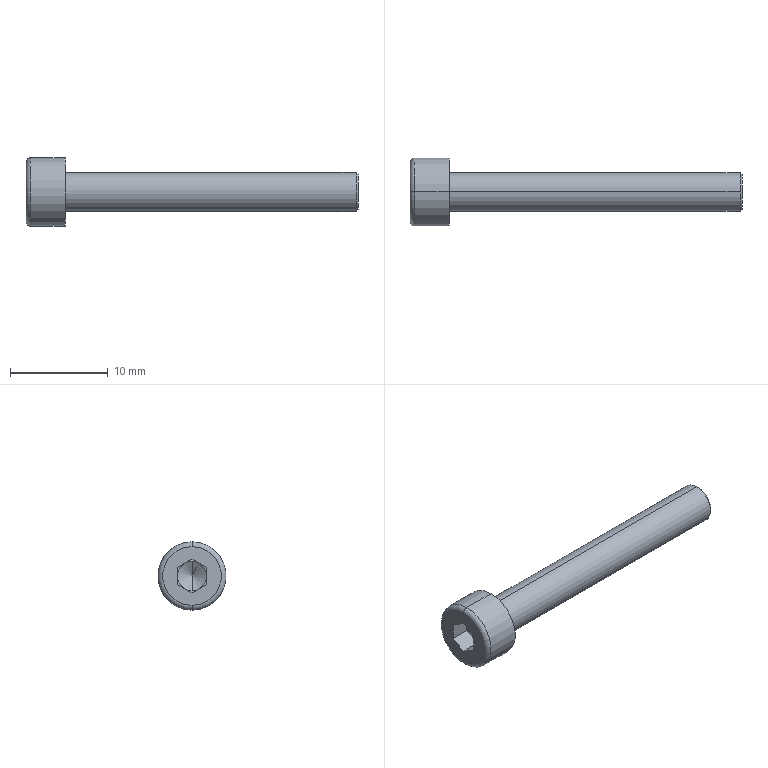Part | SolidWorks | features Fillet 2, RevCut 2, Boss 1, Chamfer 1, Cut 1, Extrusion 1, LPattern 1 | 1 solid | 25 faces | box 34 x 7 x 7 mm | volume 511.915 mm3 | plane 15 | cone 4 | cylinder 4 | torus 2 | commonest cylinder face diameters 4 x2 7 x2
STEP:
#1=CARTESIAN_POINT('',(34.,0.,-1.8));
#2=VERTEX_POINT('',#1);
#3=CARTESIAN_POINT('',(34.,0.,1.8));
#4=VERTEX_POINT('',#3);
#5=CARTESIAN_POINT('',(34.,0.,0.));
#6=DIRECTION('',(1.,0.,0.));
#7=DIRECTION('',(0.,0.,-1.));
#8=AXIS2_PLACEMENT_3D('',#5,#6,#7);
#9=CIRCLE('',#8,1.8);
#10=EDGE_CURVE('',#2,#4,#9,.T.);
#11=ORIENTED_EDGE('',*,*,#10,.F.);
#12=CARTESIAN_POINT('',(33.8,0.,-2.));
#13=VERTEX_POINT('',#12);
#14=CARTESIAN_POINT('',(34.,0.,-1.8));
#15=DIRECTION('',(-0.7071,0.,-0.7071));
#16=VECTOR('',#15,1000.);
#17=LINE('',#14,#16);
#18=EDGE_CURVE('',#2,#13,#17,.T.);
#19=ORIENTED_EDGE('',*,*,#18,.T.);
#20=CARTESIAN_POINT('',(33.8,0.,2.));
#21=VERTEX_POINT('',#20);
#22=CARTESIAN_POINT('',(33.8,0.,0.));
#23=DIRECTION('',(-1.,0.,0.));
#24=DIRECTION('',(0.,0.,-1.));
#25=AXIS2_PLACEMENT_3D('',#22,#23,#24);
#26=CIRCLE('',#25,2.);
#27=EDGE_CURVE('',#21,#13,#26,.T.);
#28=ORIENTED_EDGE('',*,*,#27,.F.);
#29=CARTESIAN_POINT('',(34.,0.,1.8));
#30=DIRECTION('',(-0.7071,0.,0.7071));
#31=VECTOR('',#30,1000.);
#32=LINE('',#29,#31);
#33=EDGE_CURVE('',#4,#21,#32,.T.);
#34=ORIENTED_EDGE('',*,*,#33,.F.);
#35=EDGE_LOOP('',(#11,#19,#28,#34));
#36=FACE_OUTER_BOUND('',#35,.T.);
#37=CARTESIAN_POINT('',(34.,0.,0.));
#38=DIRECTION('',(-1.,0.,0.));
#39=DIRECTION('',(0.,0.,1.));
#40=AXIS2_PLACEMENT_3D('',#37,#38,#39);
#41=CONICAL_SURFACE('',#40,1.8,0.7854);
#42=ADVANCED_FACE('',(#36),#41,.T.);
#43=CARTESIAN_POINT('',(0.,0.,3.));
#44=VERTEX_POINT('',#43);
#45=CARTESIAN_POINT('',(0.,0.,-3.));
#46=VERTEX_POINT('',#45);
#47=CARTESIAN_POINT('',(0.,0.,0.));
#48=DIRECTION('',(-1.,0.,0.));
#49=DIRECTION('',(0.,0.,-1.));
#50=AXIS2_PLACEMENT_3D('',#47,#48,#49);
#51=CIRCLE('',#50,3.);
#52=EDGE_CURVE('',#44,#46,#51,.T.);
#53=ORIENTED_EDGE('',*,*,#52,.F.);
#54=CARTESIAN_POINT('',(0.5,0.,3.5));
#55=VERTEX_POINT('',#54);
#56=CARTESIAN_POINT('',(0.5,0.,3.));
#57=DIRECTION('',(0.,1.,0.));
#58=DIRECTION('',(0.,0.,1.));
#59=AXIS2_PLACEMENT_3D('',#56,#57,#58);
#60=CIRCLE('',#59,0.5);
#61=EDGE_CURVE('',#44,#55,#60,.T.);
#62=ORIENTED_EDGE('',*,*,#61,.T.);
#63=CARTESIAN_POINT('',(0.5,0.,-3.5));
#64=VERTEX_POINT('',#63);
#65=CARTESIAN_POINT('',(0.5,0.,0.));
#66=DIRECTION('',(1.,0.,0.));
#67=DIRECTION('',(0.,0.,-1.));
#68=AXIS2_PLACEMENT_3D('',#65,#66,#67);
#69=CIRCLE('',#68,3.5);
#70=EDGE_CURVE('',#64,#55,#69,.T.);
#71=ORIENTED_EDGE('',*,*,#70,.F.);
#72=CARTESIAN_POINT('',(0.5,0.,-3.));
#73=DIRECTION('',(0.,-1.,0.));
#74=DIRECTION('',(0.,0.,-1.));
#75=AXIS2_PLACEMENT_3D('',#72,#73,#74);
#76=CIRCLE('',#75,0.5);
#77=EDGE_CURVE('',#46,#64,#76,.T.);
#78=ORIENTED_EDGE('',*,*,#77,.F.);
#79=EDGE_LOOP('',(#53,#62,#71,#78));
#80=FACE_OUTER_BOUND('',#79,.T.);
#81=CARTESIAN_POINT('',(0.5,0.,0.));
#82=DIRECTION('',(1.,0.,0.));
#83=DIRECTION('',(0.,0.,-1.));
#84=AXIS2_PLACEMENT_3D('',#81,#82,#83);
#85=TOROIDAL_SURFACE('',#84,3.,0.5);
#86=ADVANCED_FACE('',(#80),#85,.T.);
#87=CARTESIAN_POINT('',(2.866,0.,0.));
#88=VERTEX_POINT('',#87);
#89=CARTESIAN_POINT('',(2.,0.,1.5));
#90=VERTEX_POINT('',#89);
#91=CARTESIAN_POINT('',(2.,0.,1.5));
#92=DIRECTION('',(-0.5,0.,0.866));
#93=VECTOR('',#92,1000.);
#94=LINE('',#91,#93);
#95=EDGE_CURVE('',#88,#90,#94,.T.);
#96=ORIENTED_EDGE('',*,*,#95,.F.);
#97=CARTESIAN_POINT('',(2.,0.,-1.5));
#98=VERTEX_POINT('',#97);
#99=CARTESIAN_POINT('',(2.,0.,-1.5));
#100=DIRECTION('',(-0.5,0.,-0.866));
#101=VECTOR('',#100,1000.);
#102=LINE('',#99,#101);
#103=EDGE_CURVE('',#88,#98,#102,.T.);
#104=ORIENTED_EDGE('',*,*,#103,.T.);
#105=CARTESIAN_POINT('',(2.,-0.75,-1.299));
#106=VERTEX_POINT('',#105);
#107=CARTESIAN_POINT('',(2.,0.,0.));
#108=DIRECTION('',(-1.,0.,0.));
#109=DIRECTION('',(0.,0.,-1.));
#110=AXIS2_PLACEMENT_3D('',#107,#108,#109);
#111=CIRCLE('',#110,1.5);
#112=EDGE_CURVE('',#98,#106,#111,.T.);
#113=ORIENTED_EDGE('',*,*,#112,.T.);
#114=CARTESIAN_POINT('',(2.,-1.5,0.));
#115=VERTEX_POINT('',#114);
#116=CARTESIAN_POINT('',(2.,0.,0.));
#117=DIRECTION('',(-1.,0.,0.));
#118=DIRECTION('',(0.,0.,-1.));
#119=AXIS2_PLACEMENT_3D('',#116,#117,#118);
#120=CIRCLE('',#119,1.5);
#121=EDGE_CURVE('',#106,#115,#120,.T.);
#122=ORIENTED_EDGE('',*,*,#121,.T.);
#123=CARTESIAN_POINT('',(2.,-0.75,1.299));
#124=VERTEX_POINT('',#123);
#125=CARTESIAN_POINT('',(2.,0.,0.));
#126=DIRECTION('',(-1.,0.,0.));
#127=DIRECTION('',(0.,0.,-1.));
#128=AXIS2_PLACEMENT_3D('',#125,#126,#127);
#129=CIRCLE('',#128,1.5);
#130=EDGE_CURVE('',#115,#124,#129,.T.);
#131=ORIENTED_EDGE('',*,*,#130,.T.);
#132=CARTESIAN_POINT('',(2.,0.,0.));
#133=DIRECTION('',(-1.,0.,0.));
#134=DIRECTION('',(0.,0.,-1.));
#135=AXIS2_PLACEMENT_3D('',#132,#133,#134);
#136=CIRCLE('',#135,1.5);
#137=EDGE_CURVE('',#124,#90,#136,.T.);
#138=ORIENTED_EDGE('',*,*,#137,.T.);
#139=EDGE_LOOP('',(#96,#104,#113,#122,#131,#138));
#140=FACE_OUTER_BOUND('',#139,.T.);
#141=CARTESIAN_POINT('',(2.,0.,0.));
#142=DIRECTION('',(-1.,0.,0.));
#143=DIRECTION('',(0.,0.,1.));
#144=AXIS2_PLACEMENT_3D('',#141,#142,#143);
#145=CONICAL_SURFACE('',#144,1.5,1.047);
#146=ADVANCED_FACE('',(#140),#145,.F.);
#147=ORIENTED_EDGE('',*,*,#27,.T.);
#148=CARTESIAN_POINT('',(4.,0.,-2.));
#149=VERTEX_POINT('',#148);
#150=CARTESIAN_POINT('',(34.,0.,-2.));
#151=DIRECTION('',(-1.,0.,0.));
#152=VECTOR('',#151,1000.);
#153=LINE('',#150,#152);
#154=EDGE_CURVE('',#13,#149,#153,.T.);
#155=ORIENTED_EDGE('',*,*,#154,.T.);
#156=CARTESIAN_POINT('',(4.,0.,2.));
#157=VERTEX_POINT('',#156);
#158=CARTESIAN_POINT('',(4.,0.,0.));
#159=DIRECTION('',(1.,0.,0.));
#160=DIRECTION('',(0.,0.,-1.));
#161=AXIS2_PLACEMENT_3D('',#158,#159,#160);
#162=CIRCLE('',#161,2.);
#163=EDGE_CURVE('',#149,#157,#162,.T.);
#164=ORIENTED_EDGE('',*,*,#163,.T.);
#165=CARTESIAN_POINT('',(34.,0.,2.));
#166=DIRECTION('',(-1.,0.,0.));
#167=VECTOR('',#166,1000.);
#168=LINE('',#165,#167);
#169=EDGE_CURVE('',#21,#157,#168,.T.);
#170=ORIENTED_EDGE('',*,*,#169,.F.);
#171=EDGE_LOOP('',(#147,#155,#164,#170));
#172=FACE_OUTER_BOUND('',#171,.T.);
#173=CARTESIAN_POINT('',(34.,0.,0.));
#174=DIRECTION('',(-1.,0.,0.));
#175=DIRECTION('',(0.,0.,1.));
#176=AXIS2_PLACEMENT_3D('',#173,#174,#175);
#177=CYLINDRICAL_SURFACE('',#176,2.);
#178=ADVANCED_FACE('',(#172),#177,.T.);
#179=CARTESIAN_POINT('',(4.,0.,-3.5));
#180=VERTEX_POINT('',#179);
#181=CARTESIAN_POINT('',(4.,0.,3.5));
#182=VERTEX_POINT('',#181);
#183=CARTESIAN_POINT('',(4.,0.,0.));
#184=DIRECTION('',(1.,0.,0.));
#185=DIRECTION('',(0.,0.,-1.));
#186=AXIS2_PLACEMENT_3D('',#183,#184,#185);
#187=CIRCLE('',#186,3.5);
#188=EDGE_CURVE('',#180,#182,#187,.T.);
#189=ORIENTED_EDGE('',*,*,#188,.F.);
#190=CARTESIAN_POINT('',(4.,0.,-3.5));
#191=DIRECTION('',(-1.,0.,0.));
#192=VECTOR('',#191,1000.);
#193=LINE('',#190,#192);
#194=EDGE_CURVE('',#180,#64,#193,.T.);
#195=ORIENTED_EDGE('',*,*,#194,.T.);
#196=ORIENTED_EDGE('',*,*,#70,.T.);
#197=CARTESIAN_POINT('',(4.,0.,3.5));
#198=DIRECTION('',(-1.,0.,0.));
#199=VECTOR('',#198,1000.);
#200=LINE('',#197,#199);
#201=EDGE_CURVE('',#182,#55,#200,.T.);
#202=ORIENTED_EDGE('',*,*,#201,.F.);
#203=EDGE_LOOP('',(#189,#195,#196,#202));
#204=FACE_OUTER_BOUND('',#203,.T.);
#205=CARTESIAN_POINT('',(4.,0.,0.));
#206=DIRECTION('',(-1.,0.,0.));
#207=DIRECTION('',(0.,0.,1.));
#208=AXIS2_PLACEMENT_3D('',#205,#206,#207);
#209=CYLINDRICAL_SURFACE('',#208,3.5);
#210=ADVANCED_FACE('',(#204),#209,.T.);
#211=ORIENTED_EDGE('',*,*,#121,.F.);
#212=CARTESIAN_POINT('',(2.,-1.5,-0.866));
#213=VERTEX_POINT('',#212);
#214=CARTESIAN_POINT('',(2.,-1.5,-0.866));
#215=DIRECTION('',(0.,0.866,-0.5));
#216=VECTOR('',#215,1000.);
#217=LINE('',#214,#216);
#218=EDGE_CURVE('',#213,#106,#217,.T.);
#219=ORIENTED_EDGE('',*,*,#218,.F.);
#220=CARTESIAN_POINT('',(2.,-1.5,0.866));
#221=DIRECTION('',(0.,0.,-1.));
#222=VECTOR('',#221,1000.);
#223=LINE('',#220,#222);
#224=EDGE_CURVE('',#115,#213,#223,.T.);
#225=ORIENTED_EDGE('',*,*,#224,.F.);
#226=EDGE_LOOP('',(#211,#219,#225));
#227=FACE_OUTER_BOUND('',#226,.T.);
#228=CARTESIAN_POINT('',(2.,0.,-1.732));
#229=DIRECTION('',(1.,0.,0.));
#230=DIRECTION('',(0.,0.,-1.));
#231=AXIS2_PLACEMENT_3D('',#228,#229,#230);
#232=PLANE('',#231);
#233=ADVANCED_FACE('',(#227),#232,.F.);
#234=ORIENTED_EDGE('',*,*,#130,.F.);
#235=CARTESIAN_POINT('',(2.,-1.5,0.866));
#236=VERTEX_POINT('',#235);
#237=CARTESIAN_POINT('',(2.,-1.5,0.866));
#238=DIRECTION('',(0.,0.,-1.));
#239=VECTOR('',#238,1000.);
#240=LINE('',#237,#239);
#241=EDGE_CURVE('',#236,#115,#240,.T.);
#242=ORIENTED_EDGE('',*,*,#241,.F.);
#243=CARTESIAN_POINT('',(2.,0.,1.732));
#244=DIRECTION('',(0.,-0.866,-0.5));
#245=VECTOR('',#244,1000.);
#246=LINE('',#243,#245);
#247=EDGE_CURVE('',#124,#236,#246,.T.);
#248=ORIENTED_EDGE('',*,*,#247,.F.);
#249=EDGE_LOOP('',(#234,#242,#248));
#250=FACE_OUTER_BOUND('',#249,.T.);
#251=CARTESIAN_POINT('',(2.,0.,-1.732));
#252=DIRECTION('',(1.,0.,0.));
#253=DIRECTION('',(0.,0.,-1.));
#254=AXIS2_PLACEMENT_3D('',#251,#252,#253);
#255=PLANE('',#254);
#256=ADVANCED_FACE('',(#250),#255,.F.);
#257=ORIENTED_EDGE('',*,*,#137,.F.);
#258=CARTESIAN_POINT('',(2.,0.,1.732));
#259=VERTEX_POINT('',#258);
#260=CARTESIAN_POINT('',(2.,0.,1.732));
#261=DIRECTION('',(0.,-0.866,-0.5));
#262=VECTOR('',#261,1000.);
#263=LINE('',#260,#262);
#264=EDGE_CURVE('',#259,#124,#263,.T.);
#265=ORIENTED_EDGE('',*,*,#264,.F.);
#266=CARTESIAN_POINT('',(2.,0.75,1.299));
#267=VERTEX_POINT('',#266);
#268=CARTESIAN_POINT('',(2.,1.5,0.866));
#269=DIRECTION('',(0.,-0.866,0.5));
#270=VECTOR('',#269,1000.);
#271=LINE('',#268,#270);
#272=EDGE_CURVE('',#267,#259,#271,.T.);
#273=ORIENTED_EDGE('',*,*,#272,.F.);
#274=CARTESIAN_POINT('',(2.,0.,0.));
#275=DIRECTION('',(-1.,0.,0.));
#276=DIRECTION('',(0.,0.,-1.));
#277=AXIS2_PLACEMENT_3D('',#274,#275,#276);
#278=CIRCLE('',#277,1.5);
#279=EDGE_CURVE('',#90,#267,#278,.T.);
#280=ORIENTED_EDGE('',*,*,#279,.F.);
#281=EDGE_LOOP('',(#257,#265,#273,#280));
#282=FACE_OUTER_BOUND('',#281,.T.);
#283=CARTESIAN_POINT('',(2.,0.,-1.732));
#284=DIRECTION('',(1.,0.,0.));
#285=DIRECTION('',(0.,0.,-1.));
#286=AXIS2_PLACEMENT_3D('',#283,#284,#285);
#287=PLANE('',#286);
#288=ADVANCED_FACE('',(#282),#287,.F.);
#289=CARTESIAN_POINT('',(2.,1.5,0.));
#290=VERTEX_POINT('',#289);
#291=CARTESIAN_POINT('',(2.,0.,0.));
#292=DIRECTION('',(-1.,0.,0.));
#293=DIRECTION('',(0.,0.,-1.));
#294=AXIS2_PLACEMENT_3D('',#291,#292,#293);
#295=CIRCLE('',#294,1.5);
#296=EDGE_CURVE('',#267,#290,#295,.T.);
#297=ORIENTED_EDGE('',*,*,#296,.F.);
#298=CARTESIAN_POINT('',(2.,1.5,0.866));
#299=VERTEX_POINT('',#298);
#300=CARTESIAN_POINT('',(2.,1.5,0.866));
#301=DIRECTION('',(0.,-0.866,0.5));
#302=VECTOR('',#301,1000.);
#303=LINE('',#300,#302);
#304=EDGE_CURVE('',#299,#267,#303,.T.);
#305=ORIENTED_EDGE('',*,*,#304,.F.);
#306=CARTESIAN_POINT('',(2.,1.5,-0.866));
#307=DIRECTION('',(0.,0.,1.));
#308=VECTOR('',#307,1000.);
#309=LINE('',#306,#308);
#310=EDGE_CURVE('',#290,#299,#309,.T.);
#311=ORIENTED_EDGE('',*,*,#310,.F.);
#312=EDGE_LOOP('',(#297,#305,#311));
#313=FACE_OUTER_BOUND('',#312,.T.);
#314=CARTESIAN_POINT('',(2.,0.,-1.732));
#315=DIRECTION('',(1.,0.,0.));
#316=DIRECTION('',(0.,0.,-1.));
#317=AXIS2_PLACEMENT_3D('',#314,#315,#316);
#318=PLANE('',#317);
#319=ADVANCED_FACE('',(#313),#318,.F.);
#320=CARTESIAN_POINT('',(2.,0.75,-1.299));
#321=VERTEX_POINT('',#320);
#322=CARTESIAN_POINT('',(2.,0.,0.));
#323=DIRECTION('',(1.,0.,0.));
#324=DIRECTION('',(0.,0.,-1.));
#325=AXIS2_PLACEMENT_3D('',#322,#323,#324);
#326=CIRCLE('',#325,1.5);
#327=EDGE_CURVE('',#321,#290,#326,.T.);
#328=ORIENTED_EDGE('',*,*,#327,.T.);
#329=CARTESIAN_POINT('',(2.,1.5,-0.866));
#330=VERTEX_POINT('',#329);
#331=CARTESIAN_POINT('',(2.,1.5,-0.866));
#332=DIRECTION('',(0.,0.,1.));
#333=VECTOR('',#332,1000.);
#334=LINE('',#331,#333);
#335=EDGE_CURVE('',#330,#290,#334,.T.);
#336=ORIENTED_EDGE('',*,*,#335,.F.);
#337=CARTESIAN_POINT('',(2.,0.,-1.732));
#338=DIRECTION('',(0.,0.866,0.5));
#339=VECTOR('',#338,1000.);
#340=LINE('',#337,#339);
#341=EDGE_CURVE('',#321,#330,#340,.T.);
#342=ORIENTED_EDGE('',*,*,#341,.F.);
#343=EDGE_LOOP('',(#328,#336,#342));
#344=FACE_OUTER_BOUND('',#343,.T.);
#345=CARTESIAN_POINT('',(2.,0.,-1.732));
#346=DIRECTION('',(1.,0.,0.));
#347=DIRECTION('',(0.,0.,-1.));
#348=AXIS2_PLACEMENT_3D('',#345,#346,#347);
#349=PLANE('',#348);
#350=ADVANCED_FACE('',(#344),#349,.F.);
#351=CARTESIAN_POINT('',(2.,0.,0.));
#352=DIRECTION('',(-1.,0.,0.));
#353=DIRECTION('',(0.,0.,-1.));
#354=AXIS2_PLACEMENT_3D('',#351,#352,#353);
#355=CIRCLE('',#354,1.5);
#356=EDGE_CURVE('',#321,#98,#355,.T.);
#357=ORIENTED_EDGE('',*,*,#356,.F.);
#358=CARTESIAN_POINT('',(2.,0.,-1.732));
#359=VERTEX_POINT('',#358);
#360=CARTESIAN_POINT('',(2.,0.,-1.732));
#361=DIRECTION('',(0.,0.866,0.5));
#362=VECTOR('',#361,1000.);
#363=LINE('',#360,#362);
#364=EDGE_CURVE('',#359,#321,#363,.T.);
#365=ORIENTED_EDGE('',*,*,#364,.F.);
#366=CARTESIAN_POINT('',(2.,-1.5,-0.866));
#367=DIRECTION('',(0.,0.866,-0.5));
#368=VECTOR('',#367,1000.);
#369=LINE('',#366,#368);
#370=EDGE_CURVE('',#106,#359,#369,.T.);
#371=ORIENTED_EDGE('',*,*,#370,.F.);
#372=ORIENTED_EDGE('',*,*,#112,.F.);
#373=EDGE_LOOP('',(#357,#365,#371,#372));
#374=FACE_OUTER_BOUND('',#373,.T.);
#375=CARTESIAN_POINT('',(2.,0.,-1.732));
#376=DIRECTION('',(1.,0.,0.));
#377=DIRECTION('',(0.,0.,-1.));
#378=AXIS2_PLACEMENT_3D('',#375,#376,#377);
#379=PLANE('',#378);
#380=ADVANCED_FACE('',(#374),#379,.F.);
#381=CARTESIAN_POINT('',(0.,0.,0.));
#382=DIRECTION('',(-1.,0.,0.));
#383=DIRECTION('',(0.,0.,-1.));
#384=AXIS2_PLACEMENT_3D('',#381,#382,#383);
#385=CIRCLE('',#384,3.);
#386=EDGE_CURVE('',#46,#44,#385,.T.);
#387=ORIENTED_EDGE('',*,*,#386,.T.);
#388=ORIENTED_EDGE('',*,*,#52,.T.);
#389=EDGE_LOOP('',(#387,#388));
#390=FACE_OUTER_BOUND('',#389,.T.);
#391=CARTESIAN_POINT('',(0.,-1.5,-0.866));
#392=VERTEX_POINT('',#391);
#393=CARTESIAN_POINT('',(0.,0.,-1.732));
#394=VERTEX_POINT('',#393);
#395=CARTESIAN_POINT('',(0.,-1.5,-0.866));
#396=DIRECTION('',(0.,0.866,-0.5));
#397=VECTOR('',#396,1000.);
#398=LINE('',#395,#397);
#399=EDGE_CURVE('',#392,#394,#398,.T.);
#400=ORIENTED_EDGE('',*,*,#399,.T.);
#401=CARTESIAN_POINT('',(0.,1.5,-0.866));
#402=VERTEX_POINT('',#401);
#403=CARTESIAN_POINT('',(0.,0.,-1.732));
#404=DIRECTION('',(0.,0.866,0.5));
#405=VECTOR('',#404,1000.);
#406=LINE('',#403,#405);
#407=EDGE_CURVE('',#394,#402,#406,.T.);
#408=ORIENTED_EDGE('',*,*,#407,.T.);
#409=CARTESIAN_POINT('',(0.,1.5,0.866));
#410=VERTEX_POINT('',#409);
#411=CARTESIAN_POINT('',(0.,1.5,-0.866));
#412=DIRECTION('',(0.,0.,1.));
#413=VECTOR('',#412,1000.);
#414=LINE('',#411,#413);
#415=EDGE_CURVE('',#402,#410,#414,.T.);
#416=ORIENTED_EDGE('',*,*,#415,.T.);
#417=CARTESIAN_POINT('',(0.,0.,1.732));
#418=VERTEX_POINT('',#417);
#419=CARTESIAN_POINT('',(0.,1.5,0.866));
#420=DIRECTION('',(0.,-0.866,0.5));
#421=VECTOR('',#420,1000.);
#422=LINE('',#419,#421);
#423=EDGE_CURVE('',#410,#418,#422,.T.);
#424=ORIENTED_EDGE('',*,*,#423,.T.);
#425=CARTESIAN_POINT('',(0.,-1.5,0.866));
#426=VERTEX_POINT('',#425);
#427=CARTESIAN_POINT('',(0.,0.,1.732));
#428=DIRECTION('',(0.,-0.866,-0.5));
#429=VECTOR('',#428,1000.);
#430=LINE('',#427,#429);
#431=EDGE_CURVE('',#418,#426,#430,.T.);
#432=ORIENTED_EDGE('',*,*,#431,.T.);
#433=CARTESIAN_POINT('',(0.,-1.5,0.866));
#434=DIRECTION('',(0.,0.,-1.));
#435=VECTOR('',#434,1000.);
#436=LINE('',#433,#435);
#437=EDGE_CURVE('',#426,#392,#436,.T.);
#438=ORIENTED_EDGE('',*,*,#437,.T.);
#439=EDGE_LOOP('',(#400,#408,#416,#424,#432,#438));
#440=FACE_BOUND('',#439,.T.);
#441=CARTESIAN_POINT('',(0.,0.,0.));
#442=DIRECTION('',(1.,0.,0.));
#443=DIRECTION('',(0.,0.,-1.));
#444=AXIS2_PLACEMENT_3D('',#441,#442,#443);
#445=PLANE('',#444);
#446=ADVANCED_FACE('',(#390,#440),#445,.F.);
#447=CARTESIAN_POINT('',(4.,0.,0.));
#448=DIRECTION('',(1.,0.,0.));
#449=DIRECTION('',(0.,0.,-1.));
#450=AXIS2_PLACEMENT_3D('',#447,#448,#449);
#451=CIRCLE('',#450,3.5);
#452=EDGE_CURVE('',#182,#180,#451,.T.);
#453=ORIENTED_EDGE('',*,*,#452,.T.);
#454=ORIENTED_EDGE('',*,*,#188,.T.);
#455=EDGE_LOOP('',(#453,#454));
#456=FACE_OUTER_BOUND('',#455,.T.);
#457=CARTESIAN_POINT('',(4.,0.,0.));
#458=DIRECTION('',(1.,0.,0.));
#459=DIRECTION('',(0.,0.,-1.));
#460=AXIS2_PLACEMENT_3D('',#457,#458,#459);
#461=CIRCLE('',#460,2.);
#462=EDGE_CURVE('',#157,#149,#461,.T.);
#463=ORIENTED_EDGE('',*,*,#462,.F.);
#464=ORIENTED_EDGE('',*,*,#163,.F.);
#465=EDGE_LOOP('',(#463,#464));
#466=FACE_BOUND('',#465,.T.);
#467=CARTESIAN_POINT('',(4.,0.,0.));
#468=DIRECTION('',(1.,0.,0.));
#469=DIRECTION('',(0.,0.,-1.));
#470=AXIS2_PLACEMENT_3D('',#467,#468,#469);
#471=PLANE('',#470);
#472=ADVANCED_FACE('',(#456,#466),#471,.T.);
#473=ORIENTED_EDGE('',*,*,#194,.F.);
#474=ORIENTED_EDGE('',*,*,#452,.F.);
#475=ORIENTED_EDGE('',*,*,#201,.T.);
#476=CARTESIAN_POINT('',(0.5,0.,0.));
#477=DIRECTION('',(1.,0.,0.));
#478=DIRECTION('',(0.,0.,-1.));
#479=AXIS2_PLACEMENT_3D('',#476,#477,#478);
#480=CIRCLE('',#479,3.5);
#481=EDGE_CURVE('',#55,#64,#480,.T.);
#482=ORIENTED_EDGE('',*,*,#481,.T.);
#483=EDGE_LOOP('',(#473,#474,#475,#482));
#484=FACE_OUTER_BOUND('',#483,.T.);
#485=CARTESIAN_POINT('',(4.,0.,0.));
#486=DIRECTION('',(-1.,0.,0.));
#487=DIRECTION('',(0.,0.,1.));
#488=AXIS2_PLACEMENT_3D('',#485,#486,#487);
#489=CYLINDRICAL_SURFACE('',#488,3.5);
#490=ADVANCED_FACE('',(#484),#489,.T.);
#491=ORIENTED_EDGE('',*,*,#154,.F.);
#492=CARTESIAN_POINT('',(33.8,0.,0.));
#493=DIRECTION('',(-1.,0.,0.));
#494=DIRECTION('',(0.,0.,-1.));
#495=AXIS2_PLACEMENT_3D('',#492,#493,#494);
#496=CIRCLE('',#495,2.);
#497=EDGE_CURVE('',#13,#21,#496,.T.);
#498=ORIENTED_EDGE('',*,*,#497,.T.);
#499=ORIENTED_EDGE('',*,*,#169,.T.);
#500=ORIENTED_EDGE('',*,*,#462,.T.);
#501=EDGE_LOOP('',(#491,#498,#499,#500));
#502=FACE_OUTER_BOUND('',#501,.T.);
#503=CARTESIAN_POINT('',(34.,0.,0.));
#504=DIRECTION('',(-1.,0.,0.));
#505=DIRECTION('',(0.,0.,1.));
#506=AXIS2_PLACEMENT_3D('',#503,#504,#505);
#507=CYLINDRICAL_SURFACE('',#506,2.);
#508=ADVANCED_FACE('',(#502),#507,.T.);
#509=CARTESIAN_POINT('',(34.,0.,0.));
#510=DIRECTION('',(1.,0.,0.));
#511=DIRECTION('',(0.,0.,-1.));
#512=AXIS2_PLACEMENT_3D('',#509,#510,#511);
#513=CIRCLE('',#512,1.8);
#514=EDGE_CURVE('',#4,#2,#513,.T.);
#515=ORIENTED_EDGE('',*,*,#514,.T.);
#516=ORIENTED_EDGE('',*,*,#10,.T.);
#517=EDGE_LOOP('',(#515,#516));
#518=FACE_OUTER_BOUND('',#517,.T.);
#519=CARTESIAN_POINT('',(34.,0.,0.));
#520=DIRECTION('',(1.,0.,0.));
#521=DIRECTION('',(0.,0.,-1.));
#522=AXIS2_PLACEMENT_3D('',#519,#520,#521);
#523=PLANE('',#522);
#524=ADVANCED_FACE('',(#518),#523,.T.);
#525=ORIENTED_EDGE('',*,*,#399,.F.);
#526=CARTESIAN_POINT('',(2.,-1.5,-0.866));
#527=DIRECTION('',(-1.,0.,0.));
#528=VECTOR('',#527,1000.);
#529=LINE('',#526,#528);
#530=EDGE_CURVE('',#213,#392,#529,.T.);
#531=ORIENTED_EDGE('',*,*,#530,.F.);
#532=ORIENTED_EDGE('',*,*,#218,.T.);
#533=ORIENTED_EDGE('',*,*,#370,.T.);
#534=CARTESIAN_POINT('',(2.,0.,-1.732));
#535=DIRECTION('',(-1.,0.,0.));
#536=VECTOR('',#535,1000.);
#537=LINE('',#534,#536);
#538=EDGE_CURVE('',#359,#394,#537,.T.);
#539=ORIENTED_EDGE('',*,*,#538,.T.);
#540=EDGE_LOOP('',(#525,#531,#532,#533,#539));
#541=FACE_OUTER_BOUND('',#540,.T.);
#542=CARTESIAN_POINT('',(2.,-1.5,-0.866));
#543=DIRECTION('',(0.,0.5,0.866));
#544=DIRECTION('',(0.,-0.866,0.5));
#545=AXIS2_PLACEMENT_3D('',#542,#543,#544);
#546=PLANE('',#545);
#547=ADVANCED_FACE('',(#541),#546,.T.);
#548=ORIENTED_EDGE('',*,*,#407,.F.);
#549=ORIENTED_EDGE('',*,*,#538,.F.);
#550=ORIENTED_EDGE('',*,*,#364,.T.);
#551=ORIENTED_EDGE('',*,*,#341,.T.);
#552=CARTESIAN_POINT('',(2.,1.5,-0.866));
#553=DIRECTION('',(-1.,0.,0.));
#554=VECTOR('',#553,1000.);
#555=LINE('',#552,#554);
#556=EDGE_CURVE('',#330,#402,#555,.T.);
#557=ORIENTED_EDGE('',*,*,#556,.T.);
#558=EDGE_LOOP('',(#548,#549,#550,#551,#557));
#559=FACE_OUTER_BOUND('',#558,.T.);
#560=CARTESIAN_POINT('',(2.,0.,-1.732));
#561=DIRECTION('',(0.,-0.5,0.866));
#562=DIRECTION('',(0.,-0.866,-0.5));
#563=AXIS2_PLACEMENT_3D('',#560,#561,#562);
#564=PLANE('',#563);
#565=ADVANCED_FACE('',(#559),#564,.T.);
#566=ORIENTED_EDGE('',*,*,#415,.F.);
#567=ORIENTED_EDGE('',*,*,#556,.F.);
#568=ORIENTED_EDGE('',*,*,#335,.T.);
#569=ORIENTED_EDGE('',*,*,#310,.T.);
#570=CARTESIAN_POINT('',(2.,1.5,0.866));
#571=DIRECTION('',(-1.,0.,0.));
#572=VECTOR('',#571,1000.);
#573=LINE('',#570,#572);
#574=EDGE_CURVE('',#299,#410,#573,.T.);
#575=ORIENTED_EDGE('',*,*,#574,.T.);
#576=EDGE_LOOP('',(#566,#567,#568,#569,#575));
#577=FACE_OUTER_BOUND('',#576,.T.);
#578=CARTESIAN_POINT('',(2.,1.5,-0.866));
#579=DIRECTION('',(0.,-1.,0.));
#580=DIRECTION('',(0.,0.,-1.));
#581=AXIS2_PLACEMENT_3D('',#578,#579,#580);
#582=PLANE('',#581);
#583=ADVANCED_FACE('',(#577),#582,.T.);
#584=ORIENTED_EDGE('',*,*,#423,.F.);
#585=ORIENTED_EDGE('',*,*,#574,.F.);
#586=ORIENTED_EDGE('',*,*,#304,.T.);
#587=ORIENTED_EDGE('',*,*,#272,.T.);
#588=CARTESIAN_POINT('',(2.,0.,1.732));
#589=DIRECTION('',(-1.,0.,0.));
#590=VECTOR('',#589,1000.);
#591=LINE('',#588,#590);
#592=EDGE_CURVE('',#259,#418,#591,.T.);
#593=ORIENTED_EDGE('',*,*,#592,.T.);
#594=EDGE_LOOP('',(#584,#585,#586,#587,#593));
#595=FACE_OUTER_BOUND('',#594,.T.);
#596=CARTESIAN_POINT('',(2.,1.5,0.866));
#597=DIRECTION('',(0.,-0.5,-0.866));
#598=DIRECTION('',(0.,0.866,-0.5));
#599=AXIS2_PLACEMENT_3D('',#596,#597,#598);
#600=PLANE('',#599);
#601=ADVANCED_FACE('',(#595),#600,.T.);
#602=ORIENTED_EDGE('',*,*,#431,.F.);
#603=ORIENTED_EDGE('',*,*,#592,.F.);
#604=ORIENTED_EDGE('',*,*,#264,.T.);
#605=ORIENTED_EDGE('',*,*,#247,.T.);
#606=CARTESIAN_POINT('',(2.,-1.5,0.866));
#607=DIRECTION('',(-1.,0.,0.));
#608=VECTOR('',#607,1000.);
#609=LINE('',#606,#608);
#610=EDGE_CURVE('',#236,#426,#609,.T.);
#611=ORIENTED_EDGE('',*,*,#610,.T.);
#612=EDGE_LOOP('',(#602,#603,#604,#605,#611));
#613=FACE_OUTER_BOUND('',#612,.T.);
#614=CARTESIAN_POINT('',(2.,0.,1.732));
#615=DIRECTION('',(0.,0.5,-0.866));
#616=DIRECTION('',(0.,0.866,0.5));
#617=AXIS2_PLACEMENT_3D('',#614,#615,#616);
#618=PLANE('',#617);
#619=ADVANCED_FACE('',(#613),#618,.T.);
#620=ORIENTED_EDGE('',*,*,#437,.F.);
#621=ORIENTED_EDGE('',*,*,#610,.F.);
#622=ORIENTED_EDGE('',*,*,#241,.T.);
#623=ORIENTED_EDGE('',*,*,#224,.T.);
#624=ORIENTED_EDGE('',*,*,#530,.T.);
#625=EDGE_LOOP('',(#620,#621,#622,#623,#624));
#626=FACE_OUTER_BOUND('',#625,.T.);
#627=CARTESIAN_POINT('',(2.,-1.5,0.866));
#628=DIRECTION('',(0.,1.,0.));
#629=DIRECTION('',(0.,0.,1.));
#630=AXIS2_PLACEMENT_3D('',#627,#628,#629);
#631=PLANE('',#630);
#632=ADVANCED_FACE('',(#626),#631,.T.);
#633=ORIENTED_EDGE('',*,*,#103,.F.);
#634=ORIENTED_EDGE('',*,*,#95,.T.);
#635=ORIENTED_EDGE('',*,*,#279,.T.);
#636=ORIENTED_EDGE('',*,*,#296,.T.);
#637=ORIENTED_EDGE('',*,*,#327,.F.);
#638=ORIENTED_EDGE('',*,*,#356,.T.);
#639=EDGE_LOOP('',(#633,#634,#635,#636,#637,#638));
#640=FACE_OUTER_BOUND('',#639,.T.);
#641=CARTESIAN_POINT('',(2.,0.,0.));
#642=DIRECTION('',(-1.,0.,0.));
#643=DIRECTION('',(0.,0.,1.));
#644=AXIS2_PLACEMENT_3D('',#641,#642,#643);
#645=CONICAL_SURFACE('',#644,1.5,1.047);
#646=ADVANCED_FACE('',(#640),#645,.F.);
#647=ORIENTED_EDGE('',*,*,#61,.F.);
#648=ORIENTED_EDGE('',*,*,#386,.F.);
#649=ORIENTED_EDGE('',*,*,#77,.T.);
#650=ORIENTED_EDGE('',*,*,#481,.F.);
#651=EDGE_LOOP('',(#647,#648,#649,#650));
#652=FACE_OUTER_BOUND('',#651,.T.);
#653=CARTESIAN_POINT('',(0.5,0.,0.));
#654=DIRECTION('',(1.,0.,0.));
#655=DIRECTION('',(0.,0.,-1.));
#656=AXIS2_PLACEMENT_3D('',#653,#654,#655);
#657=TOROIDAL_SURFACE('',#656,3.,0.5);
#658=ADVANCED_FACE('',(#652),#657,.T.);
#659=ORIENTED_EDGE('',*,*,#18,.F.);
#660=ORIENTED_EDGE('',*,*,#514,.F.);
#661=ORIENTED_EDGE('',*,*,#33,.T.);
#662=ORIENTED_EDGE('',*,*,#497,.F.);
#663=EDGE_LOOP('',(#659,#660,#661,#662));
#664=FACE_OUTER_BOUND('',#663,.T.);
#665=CARTESIAN_POINT('',(34.,0.,0.));
#666=DIRECTION('',(-1.,0.,0.));
#667=DIRECTION('',(0.,0.,1.));
#668=AXIS2_PLACEMENT_3D('',#665,#666,#667);
#669=CONICAL_SURFACE('',#668,1.8,0.7854);
#670=ADVANCED_FACE('',(#664),#669,.T.);
#671=CLOSED_SHELL('',(#42,#86,#146,#178,#210,#233,#256,#288,#319,#350,#380,#446,#472,#490,#508,#524,#547,#565,#583,#601,#619,#632,#646,#658,#670));
#672=MANIFOLD_SOLID_BREP('',#671);
#673=CARTESIAN_POINT('',(0.,0.,0.));
#674=DIRECTION('',(0.,0.,1.));
#675=DIRECTION('',(1.,0.,0.));
#676=AXIS2_PLACEMENT_3D('',#673,#674,#675);
#677=(LENGTH_UNIT()NAMED_UNIT(*)SI_UNIT(.MILLI.,.METRE.));
#678=UNCERTAINTY_MEASURE_WITH_UNIT(LENGTH_MEASURE(0.00001),#677,'','');
#679=(NAMED_UNIT(*)PLANE_ANGLE_UNIT()SI_UNIT($,.RADIAN.));
#680=(NAMED_UNIT(*)SI_UNIT($,.STERADIAN.)SOLID_ANGLE_UNIT());
#681=(GEOMETRIC_REPRESENTATION_CONTEXT(3)GLOBAL_UNCERTAINTY_ASSIGNED_CONTEXT((#678))GLOBAL_UNIT_ASSIGNED_CONTEXT((#677,#679,#680))REPRESENTATION_CONTEXT('',''));
#682=ADVANCED_BREP_SHAPE_REPRESENTATION('',(#672,#676),#681);